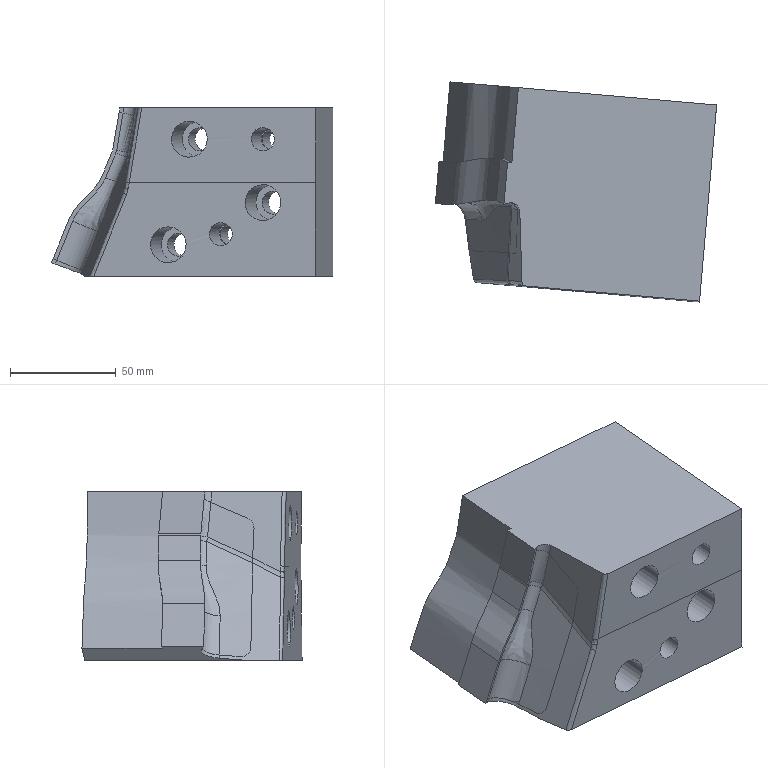Part | NX | features solid 2 | 1 solid | 49 faces | box 133.236 x 104.262 x 80 mm | volume 713678 mm3 | spline 29 | plane 10 | cylinder 10 | commonest cylinder face diameters 11 x5 17 x3 10 x2